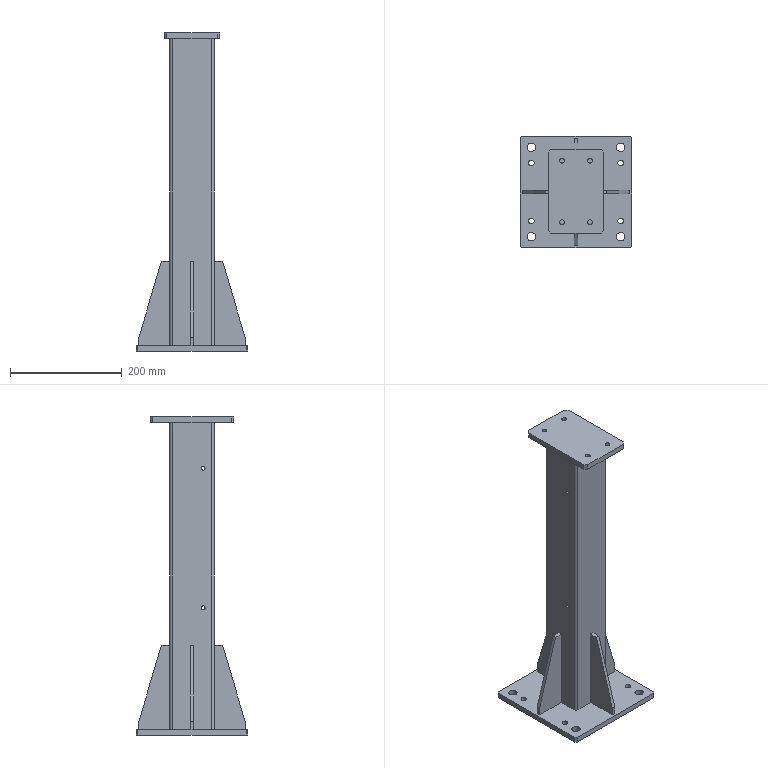Part | NX | features BREP 6 | 6 solids | 98 faces | box 200 x 200 x 570 mm | volume 1167763 mm3 | plane 58 | cylinder 40 | commonest cylinder face diameters 6.8 x8 8.5 x8 10.2 x8 15 x8 4 x4 10 x4